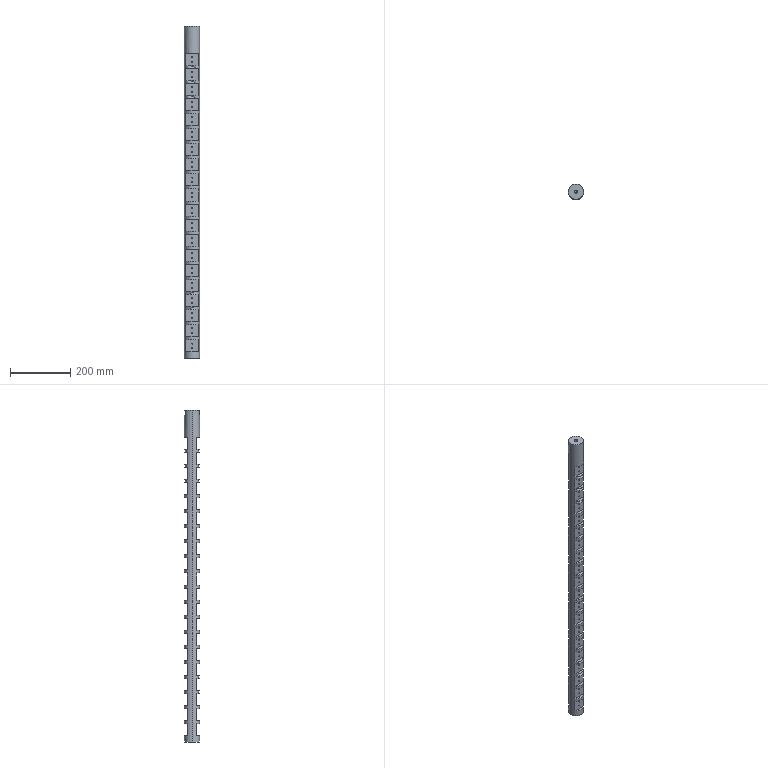Part | SolidWorks | features 3DProfileFeature 3, HoleWzd 3, ICE 2, Extrusion 1, LPattern 1, MirrorPattern 1 | 1 solid | 383 faces | box 50 x 50 x 1100 mm | volume 1552462 mm3 | cylinder 170 | plane 123 | cone 90 | commonest cylinder face diameters 3.3 x164 10.2 x2 20 x2 50 x2